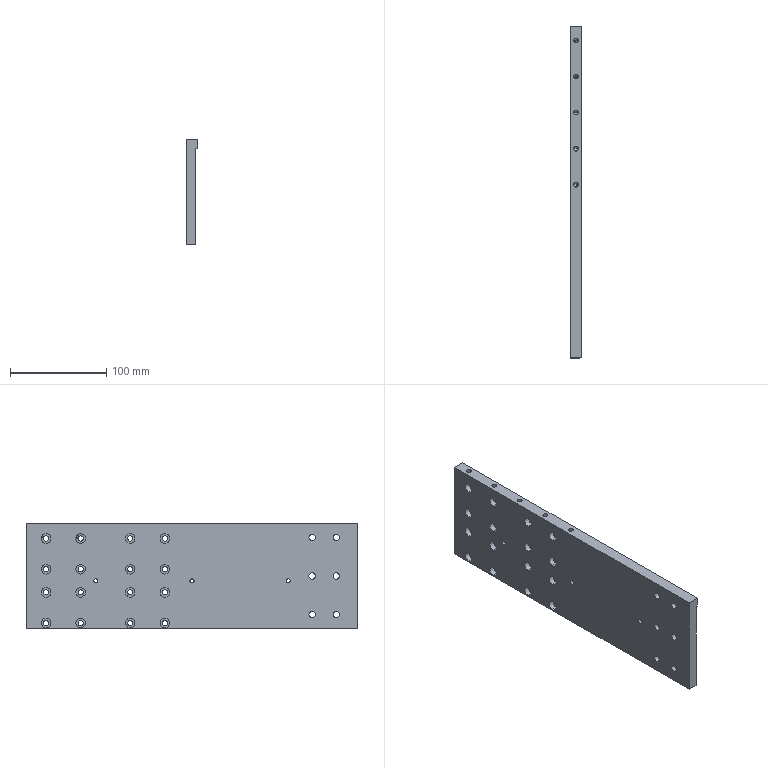Part | SolidWorks | features HoleWzd 4, Cut 1, Extrusion 1 | 1 solid | 126 faces | box 12 x 345 x 110 mm | volume 373766 mm3 | cylinder 92 | plane 24 | cone 10 | commonest cylinder face diameters 5.5 x32 10 x32 6.8 x12 5 x10 4.2 x6